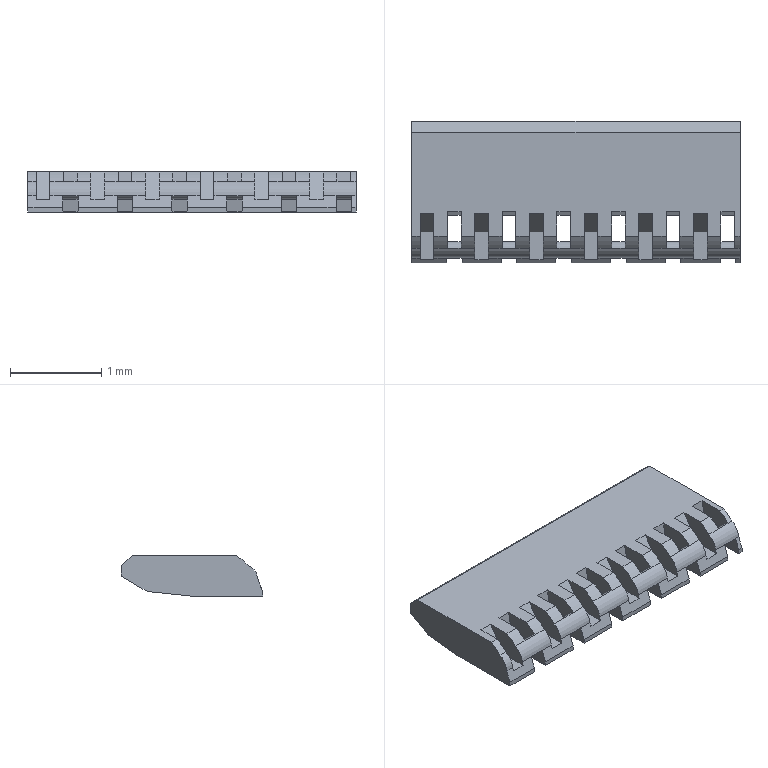Part | Creo | 1 solid | 120 faces | box 3.6 x 1.55 x 0.44 mm | volume 1.856 mm3 | plane 94 | cylinder 26 | commonest cylinder face diameters 1.165 x13 0.39 x7 0.2 x6